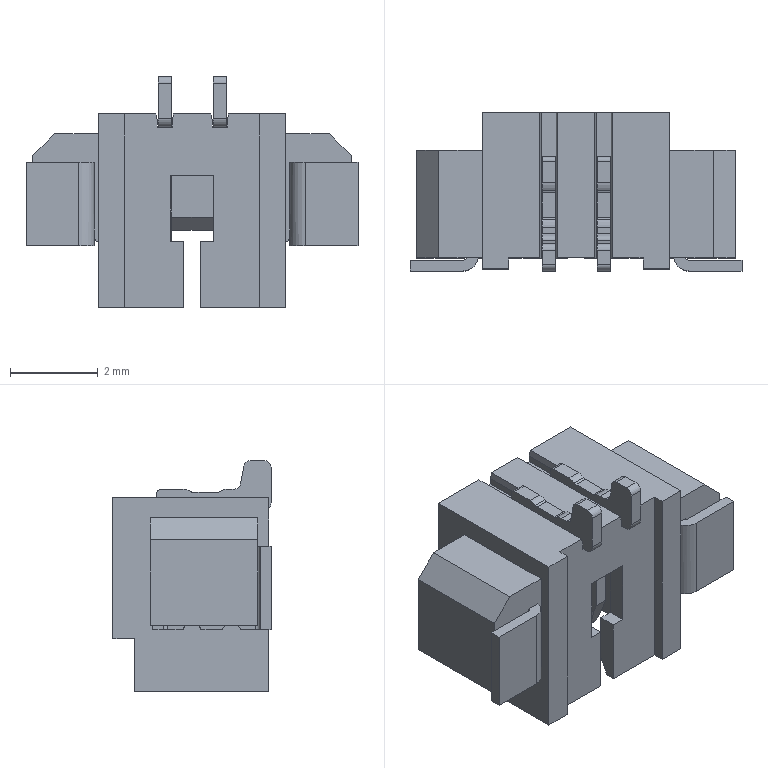Part | SolidWorks | features BaseBody 5 | 5 solids | 261 faces | box 7.55 x 3.6 x 5.25 mm | volume 54.106 mm3 | plane 191 | cylinder 70 | commonest cylinder face diameters 0.3 x30 0.2 x26 0.4 x6 0.6 x4 0.7 x4